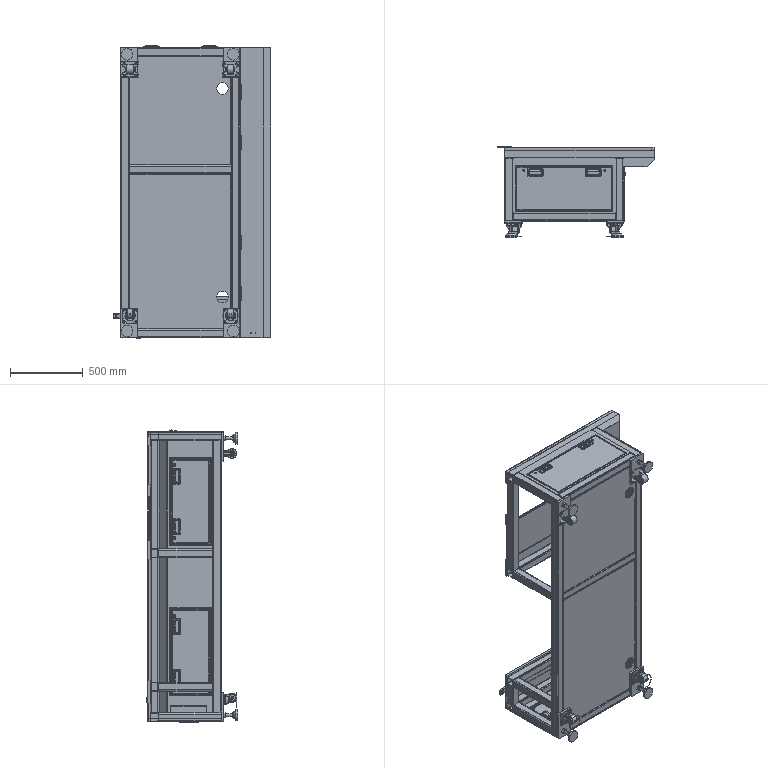Part | NX | features BREP 53 | 79 solids | 3921 faces | volume 29239912 mm3 | plane 1827 | cylinder 1473 | cone 247 | torus 222 | spline 152 | commonest cylinder face diameters 4 x148 8 x143 7 x139 10 x104 6 x94 16 x93